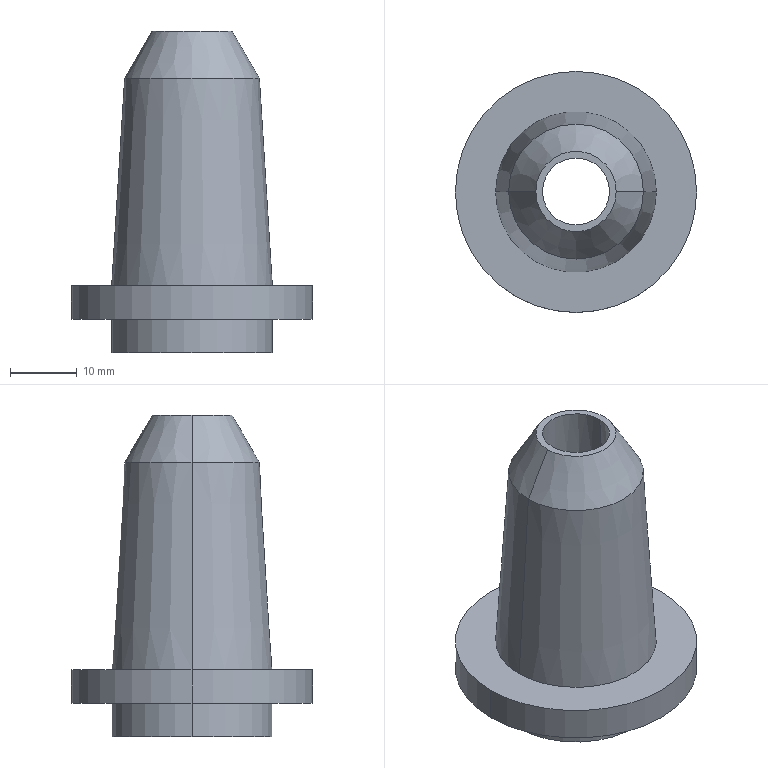Part | SolidWorks | features Extrusion 1, ICE 1, RevCut 1, Revolution 1 | 1 solid | 14 faces | box 36 x 36 x 48 mm | volume 14193 mm3 | cone 6 | cylinder 4 | plane 4 | commonest cylinder face diameters 24 x2 36 x2
STEP:
#1=CARTESIAN_POINT('',(5.,0.,48.));
#2=VERTEX_POINT('',#1);
#3=CARTESIAN_POINT('',(-5.,0.,48.));
#4=VERTEX_POINT('',#3);
#5=CARTESIAN_POINT('',(0.,0.,48.));
#6=DIRECTION('',(0.,0.,-1.));
#7=DIRECTION('',(-1.,0.,0.));
#8=AXIS2_PLACEMENT_3D('',#5,#6,#7);
#9=CIRCLE('',#8,5.);
#10=EDGE_CURVE('',#2,#4,#9,.T.);
#11=ORIENTED_EDGE('',*,*,#10,.F.);
#12=CARTESIAN_POINT('',(8.,0.,0.));
#13=VERTEX_POINT('',#12);
#14=CARTESIAN_POINT('',(5.,0.,48.));
#15=DIRECTION('',(0.06238,0.,-0.9981));
#16=VECTOR('',#15,1000.);
#17=LINE('',#14,#16);
#18=EDGE_CURVE('',#2,#13,#17,.T.);
#19=ORIENTED_EDGE('',*,*,#18,.T.);
#20=CARTESIAN_POINT('',(-8.,0.,0.));
#21=VERTEX_POINT('',#20);
#22=CARTESIAN_POINT('',(0.,0.,0.));
#23=DIRECTION('',(0.,0.,-1.));
#24=DIRECTION('',(-1.,0.,0.));
#25=AXIS2_PLACEMENT_3D('',#22,#23,#24);
#26=CIRCLE('',#25,8.);
#27=EDGE_CURVE('',#13,#21,#26,.T.);
#28=ORIENTED_EDGE('',*,*,#27,.T.);
#29=CARTESIAN_POINT('',(-5.,0.,48.));
#30=DIRECTION('',(-0.06238,0.,-0.9981));
#31=VECTOR('',#30,1000.);
#32=LINE('',#29,#31);
#33=EDGE_CURVE('',#4,#21,#32,.T.);
#34=ORIENTED_EDGE('',*,*,#33,.F.);
#35=EDGE_LOOP('',(#11,#19,#28,#34));
#36=FACE_OUTER_BOUND('',#35,.T.);
#37=CARTESIAN_POINT('',(0.,0.,48.));
#38=DIRECTION('',(0.,0.,-1.));
#39=DIRECTION('',(-1.,0.,0.));
#40=AXIS2_PLACEMENT_3D('',#37,#38,#39);
#41=CONICAL_SURFACE('',#40,5.,0.06242);
#42=ADVANCED_FACE('',(#36),#41,.F.);
#43=CARTESIAN_POINT('',(6.,0.,48.));
#44=VERTEX_POINT('',#43);
#45=CARTESIAN_POINT('',(-6.,0.,48.));
#46=VERTEX_POINT('',#45);
#47=CARTESIAN_POINT('',(0.,0.,48.));
#48=DIRECTION('',(0.,0.,1.));
#49=DIRECTION('',(1.,0.,0.));
#50=AXIS2_PLACEMENT_3D('',#47,#48,#49);
#51=CIRCLE('',#50,6.);
#52=EDGE_CURVE('',#44,#46,#51,.T.);
#53=ORIENTED_EDGE('',*,*,#52,.F.);
#54=CARTESIAN_POINT('',(10.065,0.,40.959));
#55=VERTEX_POINT('',#54);
#56=CARTESIAN_POINT('',(10.065,0.,40.959));
#57=DIRECTION('',(0.5,0.,-0.866));
#58=VECTOR('',#57,1000.);
#59=LINE('',#56,#58);
#60=EDGE_CURVE('',#44,#55,#59,.T.);
#61=ORIENTED_EDGE('',*,*,#60,.T.);
#62=CARTESIAN_POINT('',(-10.065,0.,40.959));
#63=VERTEX_POINT('',#62);
#64=CARTESIAN_POINT('',(0.,0.,40.959));
#65=DIRECTION('',(0.,0.,1.));
#66=DIRECTION('',(1.,0.,0.));
#67=AXIS2_PLACEMENT_3D('',#64,#65,#66);
#68=CIRCLE('',#67,10.065);
#69=EDGE_CURVE('',#55,#63,#68,.T.);
#70=ORIENTED_EDGE('',*,*,#69,.T.);
#71=CARTESIAN_POINT('',(-10.065,0.,40.959));
#72=DIRECTION('',(-0.5,0.,-0.866));
#73=VECTOR('',#72,1000.);
#74=LINE('',#71,#73);
#75=EDGE_CURVE('',#46,#63,#74,.T.);
#76=ORIENTED_EDGE('',*,*,#75,.F.);
#77=EDGE_LOOP('',(#53,#61,#70,#76));
#78=FACE_OUTER_BOUND('',#77,.T.);
#79=CARTESIAN_POINT('',(0.,0.,40.959));
#80=DIRECTION('',(0.,0.,-1.));
#81=DIRECTION('',(-1.,0.,0.));
#82=AXIS2_PLACEMENT_3D('',#79,#80,#81);
#83=CONICAL_SURFACE('',#82,10.065,0.5236);
#84=ADVANCED_FACE('',(#78),#83,.T.);
#85=ORIENTED_EDGE('',*,*,#69,.F.);
#86=CARTESIAN_POINT('',(12.,0.,10.));
#87=VERTEX_POINT('',#86);
#88=CARTESIAN_POINT('',(12.,0.,10.));
#89=DIRECTION('',(0.06238,0.,-0.9981));
#90=VECTOR('',#89,1000.);
#91=LINE('',#88,#90);
#92=EDGE_CURVE('',#55,#87,#91,.T.);
#93=ORIENTED_EDGE('',*,*,#92,.T.);
#94=CARTESIAN_POINT('',(-12.,0.,10.));
#95=VERTEX_POINT('',#94);
#96=CARTESIAN_POINT('',(0.,0.,10.));
#97=DIRECTION('',(0.,0.,1.));
#98=DIRECTION('',(1.,0.,0.));
#99=AXIS2_PLACEMENT_3D('',#96,#97,#98);
#100=CIRCLE('',#99,12.);
#101=EDGE_CURVE('',#87,#95,#100,.T.);
#102=ORIENTED_EDGE('',*,*,#101,.T.);
#103=CARTESIAN_POINT('',(-12.,0.,10.));
#104=DIRECTION('',(-0.06238,0.,-0.9981));
#105=VECTOR('',#104,1000.);
#106=LINE('',#103,#105);
#107=EDGE_CURVE('',#63,#95,#106,.T.);
#108=ORIENTED_EDGE('',*,*,#107,.F.);
#109=EDGE_LOOP('',(#85,#93,#102,#108));
#110=FACE_OUTER_BOUND('',#109,.T.);
#111=CARTESIAN_POINT('',(0.,0.,10.));
#112=DIRECTION('',(0.,0.,-1.));
#113=DIRECTION('',(-1.,0.,0.));
#114=AXIS2_PLACEMENT_3D('',#111,#112,#113);
#115=CONICAL_SURFACE('',#114,12.,0.06242);
#116=ADVANCED_FACE('',(#110),#115,.T.);
#117=CARTESIAN_POINT('',(18.,0.,10.));
#118=VERTEX_POINT('',#117);
#119=CARTESIAN_POINT('',(-18.,0.,10.));
#120=VERTEX_POINT('',#119);
#121=CARTESIAN_POINT('',(0.,0.,10.));
#122=DIRECTION('',(0.,0.,1.));
#123=DIRECTION('',(1.,0.,0.));
#124=AXIS2_PLACEMENT_3D('',#121,#122,#123);
#125=CIRCLE('',#124,18.);
#126=EDGE_CURVE('',#118,#120,#125,.T.);
#127=ORIENTED_EDGE('',*,*,#126,.F.);
#128=CARTESIAN_POINT('',(18.,0.,5.));
#129=VERTEX_POINT('',#128);
#130=CARTESIAN_POINT('',(18.,0.,10.));
#131=DIRECTION('',(0.,0.,-1.));
#132=VECTOR('',#131,1000.);
#133=LINE('',#130,#132);
#134=EDGE_CURVE('',#118,#129,#133,.T.);
#135=ORIENTED_EDGE('',*,*,#134,.T.);
#136=CARTESIAN_POINT('',(-18.,0.,5.));
#137=VERTEX_POINT('',#136);
#138=CARTESIAN_POINT('',(0.,0.,5.));
#139=DIRECTION('',(0.,0.,1.));
#140=DIRECTION('',(1.,0.,0.));
#141=AXIS2_PLACEMENT_3D('',#138,#139,#140);
#142=CIRCLE('',#141,18.);
#143=EDGE_CURVE('',#129,#137,#142,.T.);
#144=ORIENTED_EDGE('',*,*,#143,.T.);
#145=CARTESIAN_POINT('',(-18.,0.,10.));
#146=DIRECTION('',(0.,0.,-1.));
#147=VECTOR('',#146,1000.);
#148=LINE('',#145,#147);
#149=EDGE_CURVE('',#120,#137,#148,.T.);
#150=ORIENTED_EDGE('',*,*,#149,.F.);
#151=EDGE_LOOP('',(#127,#135,#144,#150));
#152=FACE_OUTER_BOUND('',#151,.T.);
#153=CARTESIAN_POINT('',(0.,0.,10.));
#154=DIRECTION('',(0.,0.,-1.));
#155=DIRECTION('',(-1.,0.,0.));
#156=AXIS2_PLACEMENT_3D('',#153,#154,#155);
#157=CYLINDRICAL_SURFACE('',#156,18.);
#158=ADVANCED_FACE('',(#152),#157,.T.);
#159=CARTESIAN_POINT('',(12.,0.,5.));
#160=VERTEX_POINT('',#159);
#161=CARTESIAN_POINT('',(-12.,0.,5.));
#162=VERTEX_POINT('',#161);
#163=CARTESIAN_POINT('',(0.,0.,5.));
#164=DIRECTION('',(0.,0.,1.));
#165=DIRECTION('',(1.,0.,0.));
#166=AXIS2_PLACEMENT_3D('',#163,#164,#165);
#167=CIRCLE('',#166,12.);
#168=EDGE_CURVE('',#160,#162,#167,.T.);
#169=ORIENTED_EDGE('',*,*,#168,.F.);
#170=CARTESIAN_POINT('',(12.,0.,0.));
#171=VERTEX_POINT('',#170);
#172=CARTESIAN_POINT('',(12.,0.,5.));
#173=DIRECTION('',(0.,0.,-1.));
#174=VECTOR('',#173,1000.);
#175=LINE('',#172,#174);
#176=EDGE_CURVE('',#160,#171,#175,.T.);
#177=ORIENTED_EDGE('',*,*,#176,.T.);
#178=CARTESIAN_POINT('',(-12.,0.,0.));
#179=VERTEX_POINT('',#178);
#180=CARTESIAN_POINT('',(0.,0.,0.));
#181=DIRECTION('',(0.,0.,1.));
#182=DIRECTION('',(1.,0.,0.));
#183=AXIS2_PLACEMENT_3D('',#180,#181,#182);
#184=CIRCLE('',#183,12.);
#185=EDGE_CURVE('',#171,#179,#184,.T.);
#186=ORIENTED_EDGE('',*,*,#185,.T.);
#187=CARTESIAN_POINT('',(-12.,0.,5.));
#188=DIRECTION('',(0.,0.,-1.));
#189=VECTOR('',#188,1000.);
#190=LINE('',#187,#189);
#191=EDGE_CURVE('',#162,#179,#190,.T.);
#192=ORIENTED_EDGE('',*,*,#191,.F.);
#193=EDGE_LOOP('',(#169,#177,#186,#192));
#194=FACE_OUTER_BOUND('',#193,.T.);
#195=CARTESIAN_POINT('',(0.,0.,5.));
#196=DIRECTION('',(0.,0.,-1.));
#197=DIRECTION('',(-1.,0.,0.));
#198=AXIS2_PLACEMENT_3D('',#195,#196,#197);
#199=CYLINDRICAL_SURFACE('',#198,12.);
#200=ADVANCED_FACE('',(#194),#199,.T.);
#201=ORIENTED_EDGE('',*,*,#176,.F.);
#202=CARTESIAN_POINT('',(0.,0.,5.));
#203=DIRECTION('',(0.,0.,1.));
#204=DIRECTION('',(1.,0.,0.));
#205=AXIS2_PLACEMENT_3D('',#202,#203,#204);
#206=CIRCLE('',#205,12.);
#207=EDGE_CURVE('',#162,#160,#206,.T.);
#208=ORIENTED_EDGE('',*,*,#207,.F.);
#209=ORIENTED_EDGE('',*,*,#191,.T.);
#210=CARTESIAN_POINT('',(0.,0.,0.));
#211=DIRECTION('',(0.,0.,1.));
#212=DIRECTION('',(1.,0.,0.));
#213=AXIS2_PLACEMENT_3D('',#210,#211,#212);
#214=CIRCLE('',#213,12.);
#215=EDGE_CURVE('',#179,#171,#214,.T.);
#216=ORIENTED_EDGE('',*,*,#215,.T.);
#217=EDGE_LOOP('',(#201,#208,#209,#216));
#218=FACE_OUTER_BOUND('',#217,.T.);
#219=CARTESIAN_POINT('',(0.,0.,5.));
#220=DIRECTION('',(0.,0.,-1.));
#221=DIRECTION('',(-1.,0.,0.));
#222=AXIS2_PLACEMENT_3D('',#219,#220,#221);
#223=CYLINDRICAL_SURFACE('',#222,12.);
#224=ADVANCED_FACE('',(#218),#223,.T.);
#225=CARTESIAN_POINT('',(0.,0.,0.));
#226=DIRECTION('',(0.,0.,-1.));
#227=DIRECTION('',(-1.,0.,0.));
#228=AXIS2_PLACEMENT_3D('',#225,#226,#227);
#229=CIRCLE('',#228,8.);
#230=EDGE_CURVE('',#21,#13,#229,.T.);
#231=ORIENTED_EDGE('',*,*,#230,.F.);
#232=ORIENTED_EDGE('',*,*,#27,.F.);
#233=EDGE_LOOP('',(#231,#232));
#234=FACE_BOUND('',#233,.T.);
#235=ORIENTED_EDGE('',*,*,#215,.F.);
#236=ORIENTED_EDGE('',*,*,#185,.F.);
#237=EDGE_LOOP('',(#235,#236));
#238=FACE_OUTER_BOUND('',#237,.T.);
#239=CARTESIAN_POINT('',(0.,0.,0.));
#240=DIRECTION('',(0.,0.,1.));
#241=DIRECTION('',(1.,0.,0.));
#242=AXIS2_PLACEMENT_3D('',#239,#240,#241);
#243=PLANE('',#242);
#244=ADVANCED_FACE('',(#234,#238),#243,.F.);
#245=ORIENTED_EDGE('',*,*,#134,.F.);
#246=CARTESIAN_POINT('',(0.,0.,10.));
#247=DIRECTION('',(0.,0.,1.));
#248=DIRECTION('',(1.,0.,0.));
#249=AXIS2_PLACEMENT_3D('',#246,#247,#248);
#250=CIRCLE('',#249,18.);
#251=EDGE_CURVE('',#120,#118,#250,.T.);
#252=ORIENTED_EDGE('',*,*,#251,.F.);
#253=ORIENTED_EDGE('',*,*,#149,.T.);
#254=CARTESIAN_POINT('',(0.,0.,5.));
#255=DIRECTION('',(0.,0.,1.));
#256=DIRECTION('',(1.,0.,0.));
#257=AXIS2_PLACEMENT_3D('',#254,#255,#256);
#258=CIRCLE('',#257,18.);
#259=EDGE_CURVE('',#137,#129,#258,.T.);
#260=ORIENTED_EDGE('',*,*,#259,.T.);
#261=EDGE_LOOP('',(#245,#252,#253,#260));
#262=FACE_OUTER_BOUND('',#261,.T.);
#263=CARTESIAN_POINT('',(0.,0.,10.));
#264=DIRECTION('',(0.,0.,-1.));
#265=DIRECTION('',(-1.,0.,0.));
#266=AXIS2_PLACEMENT_3D('',#263,#264,#265);
#267=CYLINDRICAL_SURFACE('',#266,18.);
#268=ADVANCED_FACE('',(#262),#267,.T.);
#269=CARTESIAN_POINT('',(0.,0.,10.));
#270=DIRECTION('',(0.,0.,1.));
#271=DIRECTION('',(1.,0.,0.));
#272=AXIS2_PLACEMENT_3D('',#269,#270,#271);
#273=CIRCLE('',#272,12.);
#274=EDGE_CURVE('',#95,#87,#273,.T.);
#275=ORIENTED_EDGE('',*,*,#274,.F.);
#276=ORIENTED_EDGE('',*,*,#101,.F.);
#277=EDGE_LOOP('',(#275,#276));
#278=FACE_BOUND('',#277,.T.);
#279=ORIENTED_EDGE('',*,*,#251,.T.);
#280=ORIENTED_EDGE('',*,*,#126,.T.);
#281=EDGE_LOOP('',(#279,#280));
#282=FACE_OUTER_BOUND('',#281,.T.);
#283=CARTESIAN_POINT('',(0.,0.,10.));
#284=DIRECTION('',(0.,0.,1.));
#285=DIRECTION('',(1.,0.,0.));
#286=AXIS2_PLACEMENT_3D('',#283,#284,#285);
#287=PLANE('',#286);
#288=ADVANCED_FACE('',(#278,#282),#287,.T.);
#289=ORIENTED_EDGE('',*,*,#207,.T.);
#290=ORIENTED_EDGE('',*,*,#168,.T.);
#291=EDGE_LOOP('',(#289,#290));
#292=FACE_BOUND('',#291,.T.);
#293=ORIENTED_EDGE('',*,*,#259,.F.);
#294=ORIENTED_EDGE('',*,*,#143,.F.);
#295=EDGE_LOOP('',(#293,#294));
#296=FACE_OUTER_BOUND('',#295,.T.);
#297=CARTESIAN_POINT('',(0.,0.,5.));
#298=DIRECTION('',(0.,0.,1.));
#299=DIRECTION('',(1.,0.,0.));
#300=AXIS2_PLACEMENT_3D('',#297,#298,#299);
#301=PLANE('',#300);
#302=ADVANCED_FACE('',(#292,#296),#301,.F.);
#303=ORIENTED_EDGE('',*,*,#92,.F.);
#304=CARTESIAN_POINT('',(0.,0.,40.959));
#305=DIRECTION('',(0.,0.,1.));
#306=DIRECTION('',(1.,0.,0.));
#307=AXIS2_PLACEMENT_3D('',#304,#305,#306);
#308=CIRCLE('',#307,10.065);
#309=EDGE_CURVE('',#63,#55,#308,.T.);
#310=ORIENTED_EDGE('',*,*,#309,.F.);
#311=ORIENTED_EDGE('',*,*,#107,.T.);
#312=ORIENTED_EDGE('',*,*,#274,.T.);
#313=EDGE_LOOP('',(#303,#310,#311,#312));
#314=FACE_OUTER_BOUND('',#313,.T.);
#315=CARTESIAN_POINT('',(0.,0.,10.));
#316=DIRECTION('',(0.,0.,-1.));
#317=DIRECTION('',(-1.,0.,0.));
#318=AXIS2_PLACEMENT_3D('',#315,#316,#317);
#319=CONICAL_SURFACE('',#318,12.,0.06242);
#320=ADVANCED_FACE('',(#314),#319,.T.);
#321=ORIENTED_EDGE('',*,*,#60,.F.);
#322=CARTESIAN_POINT('',(0.,0.,48.));
#323=DIRECTION('',(0.,0.,1.));
#324=DIRECTION('',(1.,0.,0.));
#325=AXIS2_PLACEMENT_3D('',#322,#323,#324);
#326=CIRCLE('',#325,6.);
#327=EDGE_CURVE('',#46,#44,#326,.T.);
#328=ORIENTED_EDGE('',*,*,#327,.F.);
#329=ORIENTED_EDGE('',*,*,#75,.T.);
#330=ORIENTED_EDGE('',*,*,#309,.T.);
#331=EDGE_LOOP('',(#321,#328,#329,#330));
#332=FACE_OUTER_BOUND('',#331,.T.);
#333=CARTESIAN_POINT('',(0.,0.,40.959));
#334=DIRECTION('',(0.,0.,-1.));
#335=DIRECTION('',(-1.,0.,0.));
#336=AXIS2_PLACEMENT_3D('',#333,#334,#335);
#337=CONICAL_SURFACE('',#336,10.065,0.5236);
#338=ADVANCED_FACE('',(#332),#337,.T.);
#339=CARTESIAN_POINT('',(0.,0.,48.));
#340=DIRECTION('',(0.,0.,-1.));
#341=DIRECTION('',(-1.,0.,0.));
#342=AXIS2_PLACEMENT_3D('',#339,#340,#341);
#343=CIRCLE('',#342,5.);
#344=EDGE_CURVE('',#4,#2,#343,.T.);
#345=ORIENTED_EDGE('',*,*,#344,.T.);
#346=ORIENTED_EDGE('',*,*,#10,.T.);
#347=EDGE_LOOP('',(#345,#346));
#348=FACE_BOUND('',#347,.T.);
#349=ORIENTED_EDGE('',*,*,#327,.T.);
#350=ORIENTED_EDGE('',*,*,#52,.T.);
#351=EDGE_LOOP('',(#349,#350));
#352=FACE_OUTER_BOUND('',#351,.T.);
#353=CARTESIAN_POINT('',(0.,6.,48.));
#354=DIRECTION('',(0.,0.,-1.));
#355=DIRECTION('',(-1.,0.,0.));
#356=AXIS2_PLACEMENT_3D('',#353,#354,#355);
#357=PLANE('',#356);
#358=ADVANCED_FACE('',(#348,#352),#357,.F.);
#359=ORIENTED_EDGE('',*,*,#18,.F.);
#360=ORIENTED_EDGE('',*,*,#344,.F.);
#361=ORIENTED_EDGE('',*,*,#33,.T.);
#362=ORIENTED_EDGE('',*,*,#230,.T.);
#363=EDGE_LOOP('',(#359,#360,#361,#362));
#364=FACE_OUTER_BOUND('',#363,.T.);
#365=CARTESIAN_POINT('',(0.,0.,48.));
#366=DIRECTION('',(0.,0.,-1.));
#367=DIRECTION('',(-1.,0.,0.));
#368=AXIS2_PLACEMENT_3D('',#365,#366,#367);
#369=CONICAL_SURFACE('',#368,5.,0.06242);
#370=ADVANCED_FACE('',(#364),#369,.F.);
#371=CLOSED_SHELL('',(#42,#84,#116,#158,#200,#224,#244,#268,#288,#302,#320,#338,#358,#370));
#372=MANIFOLD_SOLID_BREP('',#371);
#373=CARTESIAN_POINT('',(0.,0.,0.));
#374=DIRECTION('',(0.,0.,1.));
#375=DIRECTION('',(1.,0.,0.));
#376=AXIS2_PLACEMENT_3D('',#373,#374,#375);
#377=(LENGTH_UNIT()NAMED_UNIT(*)SI_UNIT(.MILLI.,.METRE.));
#378=UNCERTAINTY_MEASURE_WITH_UNIT(LENGTH_MEASURE(0.00001),#377,'','');
#379=(NAMED_UNIT(*)PLANE_ANGLE_UNIT()SI_UNIT($,.RADIAN.));
#380=(NAMED_UNIT(*)SI_UNIT($,.STERADIAN.)SOLID_ANGLE_UNIT());
#381=(GEOMETRIC_REPRESENTATION_CONTEXT(3)GLOBAL_UNCERTAINTY_ASSIGNED_CONTEXT((#378))GLOBAL_UNIT_ASSIGNED_CONTEXT((#377,#379,#380))REPRESENTATION_CONTEXT('',''));
#382=ADVANCED_BREP_SHAPE_REPRESENTATION('',(#372,#376),#381);